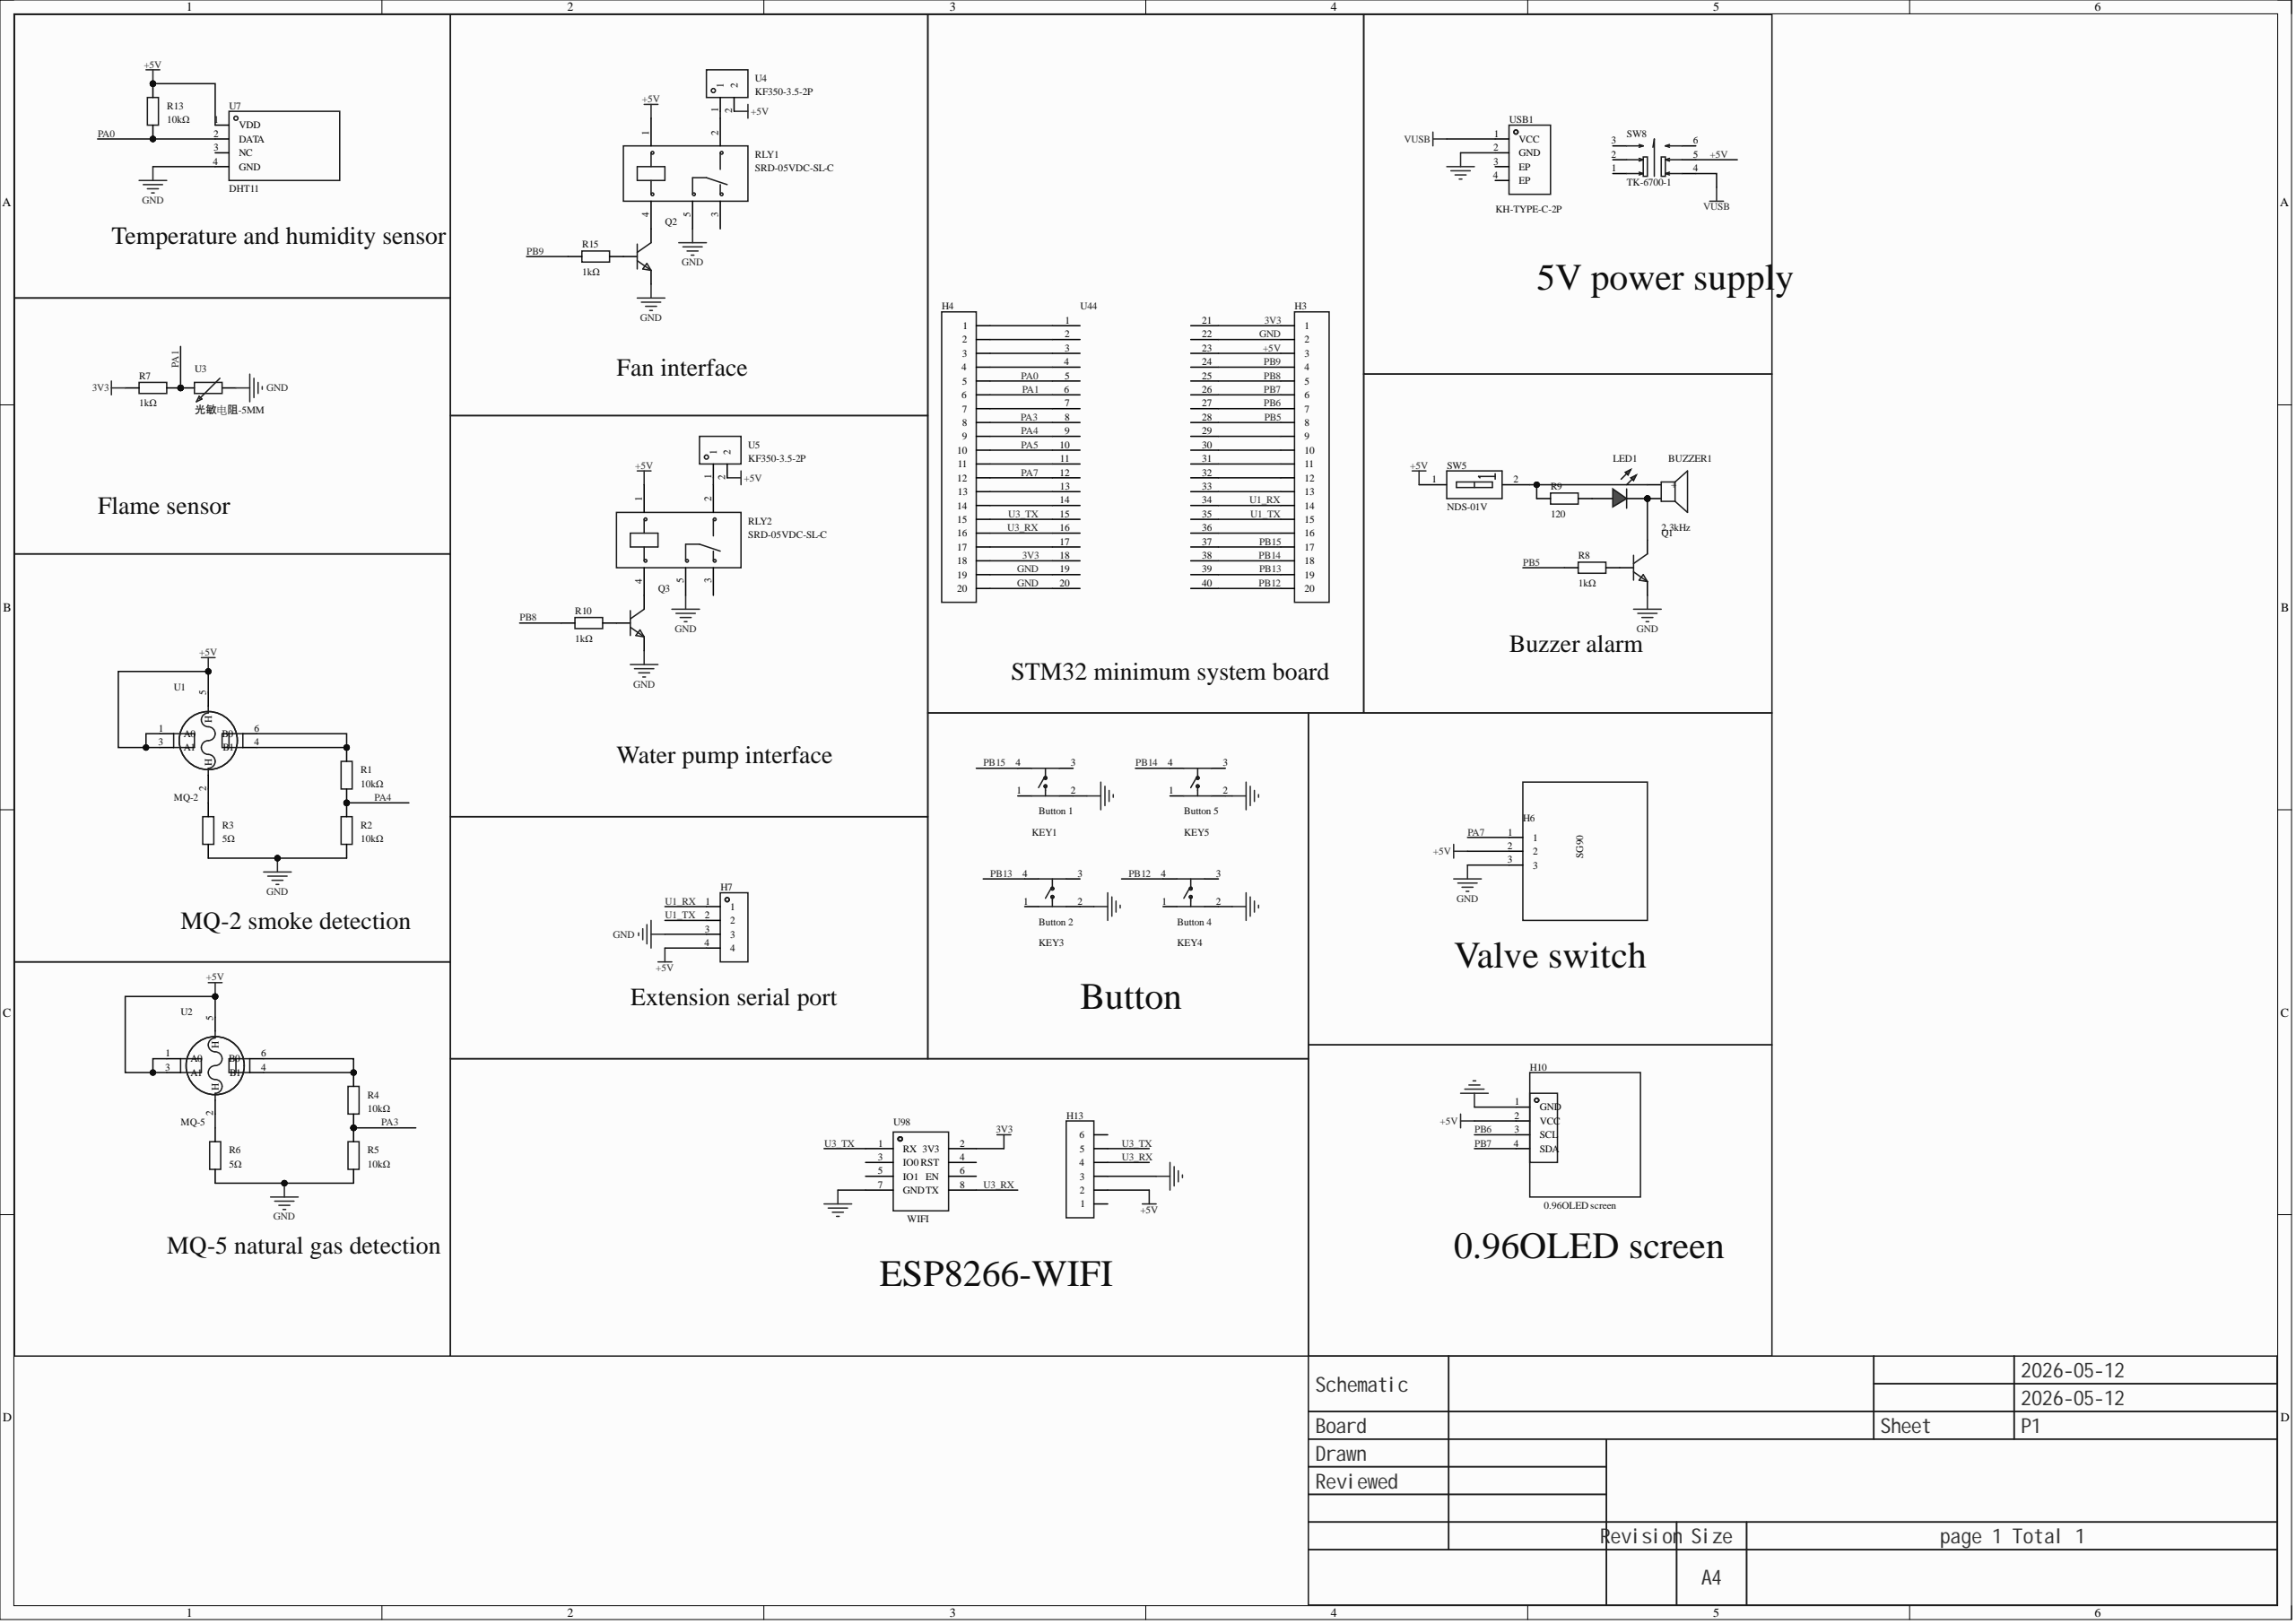Circuit board | Altium Designer | 40 parts | 52 nets
Bill of materials:
Comment,Description,Designator,Footprint,LibRef,Quantity
"2.3kHz","Drive method: active (built-in driver circuit); Construction type: electromagnetic; Rated voltage: 5V; Frequency: 2.3kHz; Sound pressure (SPL): 85dB@5V,10cm;","BUZZER1","BUZ-TH_BD12.0-P7.60-D0.6-FD","TMB12A05_C96093","1"
"","","H3, H4","HDR-TH_20P-P2.54-V-F","HDR-F_2.54_1x20P","2"
"","","H6","HDR-TH_3P-P2.54-V-F","HDR-F_2.54_1x3P","1"
"","","H7","HDR-TH_4P-P2.54-V-F","HDR-F_2.54_1x4P","1"
"2.54-1*4P female","","H10","HDR-TH_4P-P2.54-V-F","0.96OLED屏幕","1"
"","","H13","HDR-TH_6P-P2.54-V-M-1","HDR-M_2.54_1x6P","1"
"Button 1","Circuit structure: SPST; Contact rated current: -; Button head type: Round Button; Button actuation direction: Top Actuated;","KEY1","KEY-TH_4P-L6.0-W6.0-P4.50-LS7.5","按键开关6*6*8","1"
"Button 2","Circuit structure: SPST; Contact rated current: -; Button head type: Round Button; Button actuation direction: Top Actuated;","KEY3","KEY-TH_4P-L6.0-W6.0-P4.50-LS7.5","按键开关6*6*8","1"
"Button 4","Circuit structure: SPST; Contact rated current: -; Button head type: Round Button; Button actuation direction: Top Actuated;","KEY4","KEY-TH_4P-L6.0-W6.0-P4.50-LS7.5","按键开关6*6*8","1"
"Button 5","Circuit structure: SPST; Contact rated current: -; Button head type: Round Button; Button actuation direction: Top Actuated;","KEY5","KEY-TH_4P-L6.0-W6.0-P4.50-LS7.5","按键开关6*6*8","1"
"","","LED1","LED_TH-3mm","LED_TH-R_3mm","1"
"","","Q1, Q2, Q3","S8050_TO_92","S8050_TO_NPN","3"
"10kΩ","","R1, R2, R4, R5, R13","Res_1/4W","Res_AXIAL-1/8W","5"
"5Ω","","R3, R6","Res_1/4W","Res_AXIAL-1/8W","2"
"1kΩ","","R7, R8, R10, R15","Res_1/4W","Res_AXIAL-1/4W, Res_AXIAL-1/8W","4"
"120","","R9","Res_1/4W","Res_AXIAL-1/4W","1"
"SRD-05VDC-SL-C","Coil voltage: 5V; Contact form: 1C changeover (SPDT); Contact capacity (resistive load): -; Max switching voltage: 250V@AC; Max switching current: 15A;","RLY1, RLY2","RELAY-TH_SRD-XXVDC-XL-C","SRD-05VDC-SL-C","2"
"NDS-01V","Tall lever, forward action","SW5","SW-TH_2P-L3.9-W9.9-P2.54-LS7.6","NDS-01V_C501305","1"
"TK-6700-1","","SW8","SW-TH_TK-6700-1","TK-6700-1","1"
"MQ-2","","U1","SENSOR-TH_MQ-2","MQ-2","1"
"MQ-5","","U2","SENSOR-TH_MQ-2","MQ-2","1"
"光敏电阻-5MM","","U3","RES-TH_L4.9-W4.3-P3.4","光敏电阻-5MM","1"
"KF350-3.5-2P","","U4, U5","CONN-TH_P3.50_KF350-3.5-2P","KF350-3.5-2P","2"
"DHT11","","U7","SENSOR-TH_DHT11","DHT11","1"
"","","U44","STM32最小系统板","STM32最小系统板","1"
"","","U98","WiFi封装","WiFi模块","1"
"KH-TYPE-C-2P","Connector type: Type-C; Standard: -; Male/female: -; Port count: -; Contact count: 2P; Mounting: -; Rated current - power: -; Contact material: -; Contact plating: -; Operating temperature range: -;","USB1","USB-SMD_KH-TYPE-C-2P","KH-TYPE-C-2P","1"
Netlist (Protel format):
[
BUZZER1
BUZ-TH_BD12.0-P7.60-D0.6-FD
2.3kHz



]
[
H3
HDR-TH_20P-P2.54-V-F




]
[
H4
HDR-TH_20P-P2.54-V-F




]
[
H6
HDR-TH_3P-P2.54-V-F




]
[
H7
HDR-TH_4P-P2.54-V-F




]
[
H10
HDR-TH_4P-P2.54-V-F
2.54-1*4P female



]
[
H13
HDR-TH_6P-P2.54-V-M-1




]
[
KEY1
KEY-TH_4P-L6.0-W6.0-P4.50-LS7.5
Button 1



]
[
KEY3
KEY-TH_4P-L6.0-W6.0-P4.50-LS7.5
Button 2



]
[
KEY4
KEY-TH_4P-L6.0-W6.0-P4.50-LS7.5
Button 4



]
[
KEY5
KEY-TH_4P-L6.0-W6.0-P4.50-LS7.5
Button 5



]
[
LED1
LED_TH-3mm




]
[
Q1
S8050_TO_92




]
[
Q2
S8050_TO_92




]
[
Q3
S8050_TO_92




]
[
R1
Res_1/4W
10kΩ



]
[
R2
Res_1/4W
10kΩ



]
[
R3
Res_1/4W
5Ω



]
[
R4
Res_1/4W
10kΩ



]
[
R5
Res_1/4W
10kΩ



]
[
R6
Res_1/4W
5Ω



]
[
R7
Res_1/4W
1kΩ



]
[
R8
Res_1/4W
1kΩ



]
[
R9
Res_1/4W
120



]
[
R10
Res_1/4W
1kΩ



]
[
R13
Res_1/4W
10kΩ



]
[
R15
Res_1/4W
1kΩ



]
[
RLY1
RELAY-TH_SRD-XXVDC-XL-C
SRD-05VDC-SL-C



]
[
RLY2
RELAY-TH_SRD-XXVDC-XL-C
SRD-05VDC-SL-C



]
[
SW5
SW-TH_2P-L3.9-W9.9-P2.54-LS7.6
NDS-01V



]
[
SW8
SW-TH_TK-6700-1
TK-6700-1



]
[
U1
SENSOR-TH_MQ-2
MQ-2



]
[
U2
SENSOR-TH_MQ-2
MQ-5



]
[
U3
RES-TH_L4.9-W4.3-P3.4
光敏电阻-5MM



]
[
U4
CONN-TH_P3.50_KF350-3.5-2P
KF350-3.5-2P



]
[
U5
CONN-TH_P3.50_KF350-3.5-2P
KF350-3.5-2P



]
[
U7
SENSOR-TH_DHT11
DHT11



]
[
U44
STM32最小系统板




]
[
U98
WiFi封装




]
[
USB1
USB-SMD_KH-TYPE-C-2P
KH-TYPE-C-2P



]
(
VUSB
SW8-4
USB1-1
)
(
U3_TX
H4-15
H13-5
U44-15
U98-1
)
(
U3_RX
H4-16
H13-4
U44-16
U98-8
)
(
U1_TX
H3-15
H7-2
U44-35
)
(
U1_RX
H3-14
H7-1
U44-34
)
(
PB15
H3-17
KEY1-4
U44-37
)
(
PB14
H3-18
KEY5-4
U44-38
)
(
PB13
H3-19
KEY3-4
U44-39
)
(
PB12
H3-20
KEY4-4
U44-40
)
(
PB9
H3-4
R15-1
U44-24
)
(
PB8
H3-5
R10-1
U44-25
)
(
PB7
H3-6
H10-4
U44-26
)
(
PB6
H3-7
H10-3
U44-27
)
(
PB5
H3-8
R8-1
U44-28
)
(
PA7
H4-12
H6-1
U44-12
)
(
PA5
H4-10
U44-10
)
(
PA4
H4-9
R1-1
R2-2
U44-9
)
(
PA3
H4-8
R4-1
R5-2
U44-8
)
(
PA1
H4-6
R7-2
U3-2
U44-6
)
(
PA0
H4-5
R13-1
U7-2
U44-5
)
(
NetRLY2_2
RLY2-2
U5-1
)
(
NetRLY1_2
RLY1-2
U4-1
)
(
NetR6_2
R6-2
U2-2
)
(
NetR4_2
R4-2
U2-4
U2-6
)
(
NetR3_2
R3-2
U1-2
)
(
NetR1_2
R1-2
U1-4
U1-6
)
(
NetQ3_3
Q3-3
RLY2-4
)
(
NetQ3_2
Q3-2
R10-2
)
(
NetQ2_3
Q2-3
RLY1-4
)
(
NetQ2_2
Q2-2
R15-2
)
(
NetQ1_2
Q1-2
R8-2
)
(
NetLED1_1
LED1-1
R9-2
)
(
NetH4_17
H4-17
U44-17
)
(
NetH4_14
H4-14
U44-14
)
(
NetH4_13
H4-13
U44-13
)
(
NetH4_11
H4-11
U44-11
)
(
NetH4_7
H4-7
U44-7
)
(
NetH4_4
H4-4
U44-4
)
(
NetH4_3
H4-3
U44-3
)
(
NetH4_2
H4-2
U44-2
)
(
NetH4_1
H4-1
U44-1
)
(
NetH3_16
H3-16
U44-36
)
(
NetH3_13
H3-13
U44-33
)
(
NetH3_12
H3-12
U44-32
)
(
NetH3_11
H3-11
U44-31
)
(
NetH3_10
H3-10
U44-30
)
(
NetH3_9
H3-9
U44-29
)
(
NetBUZZER1_2
BUZZER1-2
LED1-2
Q1-3
)
(
NetBUZZER1_1
BUZZER1-1
R9-1
SW5-2
)
(
GND
H3-2
H4-19
H4-20
H6-3
H7-3
H10-1
H13-3
KEY1-2
KEY3-2
KEY4-2
KEY5-2
Q1-1
Q2-1
Q3-1
R2-1
R3-1
R5-1
R6-1
RLY1-5
RLY2-5
U3-1
U7-4
U44-19
U44-20
U44-22
U98-7
USB1-2
)
(
+5V
H3-3
H6-2
H7-4
H10-2
H13-2
R13-2
RLY1-1
RLY2-1
SW5-1
SW8-5
U1-1
U1-3
U1-5
U2-1
U2-3
U2-5
U4-2
U5-2
U7-1
U44-23
)
(
3V3
H3-1
H4-18
R7-1
U44-18
U44-21
U98-2
)